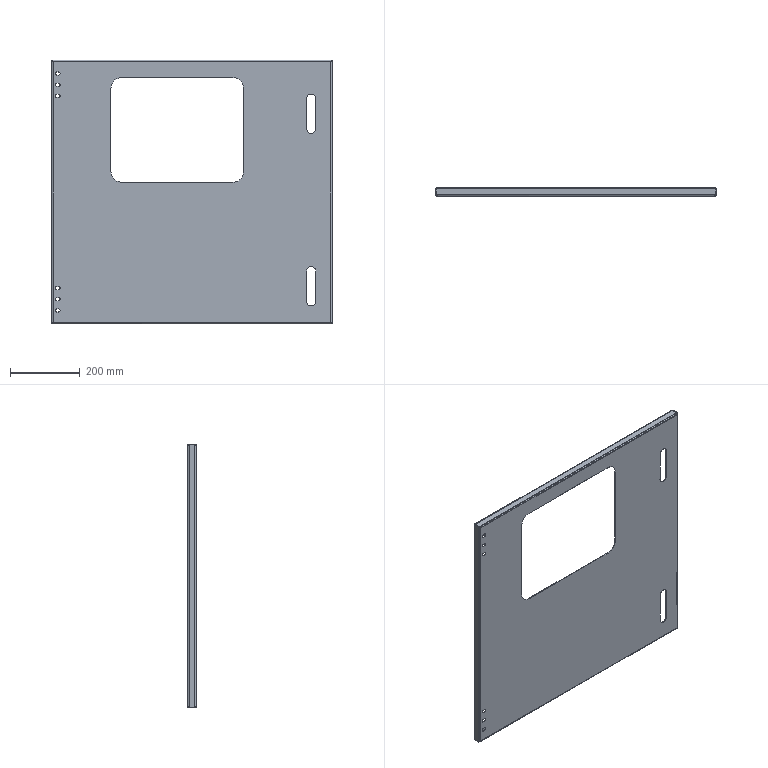Part | SolidWorks | features CornerFeat 4, ICE 4, EdgeFlange 2, Fillet 2, FlatPattern 1, SMBaseFlange 1, SheetMetal 1 | 1 solid | 132 faces | box 805 x 25 x 756 mm | volume 1238961 mm3 | plane 66 | cylinder 50 | spline 16 | commonest cylinder face diameters 9 x18 4 x8 8 x8 6 x4 10 x4 26.5 x4